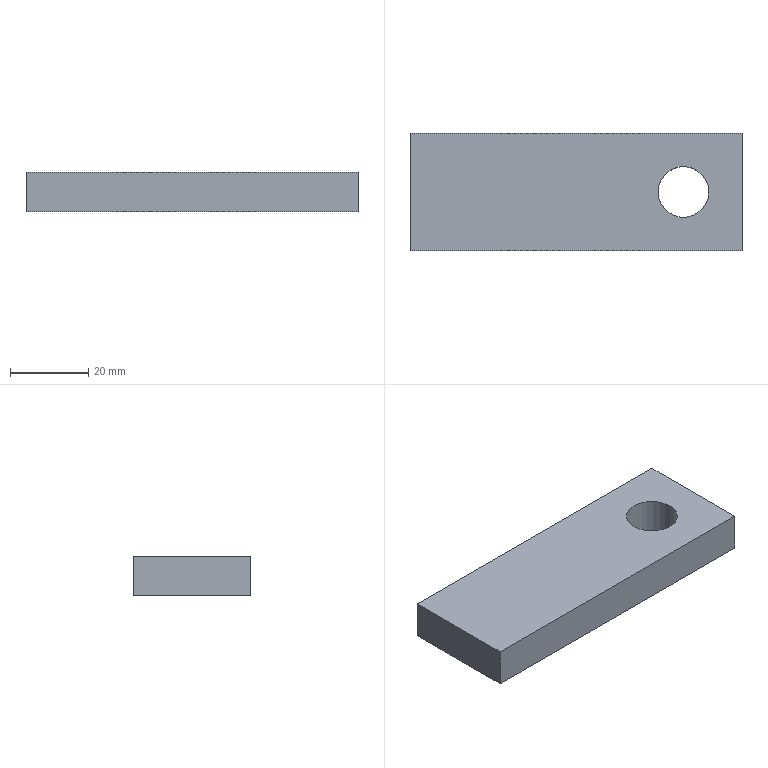Part | NX | features solid 2 | 1 solid | 7 faces | box 85 x 30 x 10 mm | volume 24173 mm3 | plane 6 | cylinder 1 | commonest cylinder face diameters 13 x1
STEP:
#1=CARTESIAN_POINT('',(-510.,-55.,-65.));
#2=VERTEX_POINT('',#1);
#3=CARTESIAN_POINT('',(-510.,-55.,-55.));
#4=VERTEX_POINT('',#3);
#5=CARTESIAN_POINT('',(-510.,-55.,0.));
#6=DIRECTION('',(0.,0.,-1.));
#7=VECTOR('',#6,1000.);
#8=LINE('',#5,#7);
#9=EDGE_CURVE('',#2,#4,#8,.F.);
#10=ORIENTED_EDGE('',*,*,#9,.T.);
#11=CARTESIAN_POINT('',(-595.,-55.,-55.));
#12=VERTEX_POINT('',#11);
#13=CARTESIAN_POINT('',(-610.,-55.,-55.));
#14=DIRECTION('',(-1.,0.,0.));
#15=VECTOR('',#14,1000.);
#16=LINE('',#13,#15);
#17=EDGE_CURVE('',#4,#12,#16,.T.);
#18=ORIENTED_EDGE('',*,*,#17,.T.);
#19=CARTESIAN_POINT('',(-595.,-55.,-65.));
#20=VERTEX_POINT('',#19);
#21=CARTESIAN_POINT('',(-595.,-55.,-65.));
#22=DIRECTION('',(0.,0.,-1.));
#23=VECTOR('',#22,1000.);
#24=LINE('',#21,#23);
#25=EDGE_CURVE('',#12,#20,#24,.T.);
#26=ORIENTED_EDGE('',*,*,#25,.T.);
#27=CARTESIAN_POINT('',(-610.,-55.,-65.));
#28=DIRECTION('',(-1.,0.,0.));
#29=VECTOR('',#28,1000.);
#30=LINE('',#27,#29);
#31=EDGE_CURVE('',#20,#2,#30,.F.);
#32=ORIENTED_EDGE('',*,*,#31,.T.);
#33=EDGE_LOOP('',(#10,#18,#26,#32));
#34=FACE_BOUND('',#33,.T.);
#35=CARTESIAN_POINT('',(-525.,-55.,0.));
#36=DIRECTION('',(0.,-1.,0.));
#37=DIRECTION('',(0.,0.,-1.));
#38=AXIS2_PLACEMENT_3D('',#35,#36,#37);
#39=PLANE('',#38);
#40=ADVANCED_FACE('',(#34),#39,.T.);
#41=CARTESIAN_POINT('',(-531.5,-40.,-55.));
#42=VERTEX_POINT('',#41);
#43=CARTESIAN_POINT('',(-525.,-40.,-55.));
#44=DIRECTION('',(0.,0.,-1.));
#45=DIRECTION('',(-1.,0.,0.));
#46=AXIS2_PLACEMENT_3D('',#43,#44,#45);
#47=CIRCLE('',#46,6.5);
#48=EDGE_CURVE('',#42,#42,#47,.T.);
#49=ORIENTED_EDGE('',*,*,#48,.F.);
#50=EDGE_LOOP('',(#49));
#51=FACE_BOUND('',#50,.T.);
#52=CARTESIAN_POINT('',(-531.5,-40.,-65.));
#53=VERTEX_POINT('',#52);
#54=CARTESIAN_POINT('',(-525.,-40.,-65.));
#55=DIRECTION('',(0.,0.,-1.));
#56=DIRECTION('',(-1.,0.,0.));
#57=AXIS2_PLACEMENT_3D('',#54,#55,#56);
#58=CIRCLE('',#57,6.5);
#59=EDGE_CURVE('',#53,#53,#58,.F.);
#60=ORIENTED_EDGE('',*,*,#59,.F.);
#61=EDGE_LOOP('',(#60));
#62=FACE_BOUND('',#61,.T.);
#63=CARTESIAN_POINT('',(-525.,-40.,-55.));
#64=DIRECTION('',(0.,0.,-1.));
#65=DIRECTION('',(-1.,0.,0.));
#66=AXIS2_PLACEMENT_3D('',#63,#64,#65);
#67=CYLINDRICAL_SURFACE('',#66,6.5);
#68=ADVANCED_FACE('',(#51,#62),#67,.F.);
#69=CARTESIAN_POINT('',(-595.,-25.,-65.));
#70=VERTEX_POINT('',#69);
#71=CARTESIAN_POINT('',(-510.,-25.,-65.));
#72=VERTEX_POINT('',#71);
#73=CARTESIAN_POINT('',(-610.,-25.,-65.));
#74=DIRECTION('',(-1.,0.,0.));
#75=VECTOR('',#74,1000.);
#76=LINE('',#73,#75);
#77=EDGE_CURVE('',#70,#72,#76,.F.);
#78=ORIENTED_EDGE('',*,*,#77,.F.);
#79=CARTESIAN_POINT('',(-595.,-25.,-55.));
#80=VERTEX_POINT('',#79);
#81=CARTESIAN_POINT('',(-595.,-25.,-65.));
#82=DIRECTION('',(0.,0.,1.));
#83=VECTOR('',#82,1000.);
#84=LINE('',#81,#83);
#85=EDGE_CURVE('',#70,#80,#84,.T.);
#86=ORIENTED_EDGE('',*,*,#85,.T.);
#87=CARTESIAN_POINT('',(-510.,-25.,-55.));
#88=VERTEX_POINT('',#87);
#89=CARTESIAN_POINT('',(-610.,-25.,-55.));
#90=DIRECTION('',(-1.,0.,0.));
#91=VECTOR('',#90,1000.);
#92=LINE('',#89,#91);
#93=EDGE_CURVE('',#88,#80,#92,.T.);
#94=ORIENTED_EDGE('',*,*,#93,.F.);
#95=CARTESIAN_POINT('',(-510.,-25.,0.));
#96=DIRECTION('',(0.,0.,1.));
#97=VECTOR('',#96,1000.);
#98=LINE('',#95,#97);
#99=EDGE_CURVE('',#88,#72,#98,.F.);
#100=ORIENTED_EDGE('',*,*,#99,.T.);
#101=EDGE_LOOP('',(#78,#86,#94,#100));
#102=FACE_BOUND('',#101,.T.);
#103=CARTESIAN_POINT('',(-525.,-25.,0.));
#104=DIRECTION('',(0.,-1.,0.));
#105=DIRECTION('',(0.,0.,-1.));
#106=AXIS2_PLACEMENT_3D('',#103,#104,#105);
#107=PLANE('',#106);
#108=ADVANCED_FACE('',(#102),#107,.F.);
#109=ORIENTED_EDGE('',*,*,#85,.F.);
#110=CARTESIAN_POINT('',(-595.,110.,-65.));
#111=DIRECTION('',(0.,1.,0.));
#112=VECTOR('',#111,1000.);
#113=LINE('',#110,#112);
#114=EDGE_CURVE('',#20,#70,#113,.T.);
#115=ORIENTED_EDGE('',*,*,#114,.F.);
#116=ORIENTED_EDGE('',*,*,#25,.F.);
#117=CARTESIAN_POINT('',(-595.,110.,-55.));
#118=DIRECTION('',(0.,1.,0.));
#119=VECTOR('',#118,1000.);
#120=LINE('',#117,#119);
#121=EDGE_CURVE('',#12,#80,#120,.T.);
#122=ORIENTED_EDGE('',*,*,#121,.T.);
#123=EDGE_LOOP('',(#109,#115,#116,#122));
#124=FACE_BOUND('',#123,.T.);
#125=CARTESIAN_POINT('',(-595.,110.,-65.));
#126=DIRECTION('',(1.,0.,0.));
#127=DIRECTION('',(0.,0.,-1.));
#128=AXIS2_PLACEMENT_3D('',#125,#126,#127);
#129=PLANE('',#128);
#130=ADVANCED_FACE('',(#124),#129,.F.);
#131=ORIENTED_EDGE('',*,*,#9,.F.);
#132=CARTESIAN_POINT('',(-510.,90.,-65.));
#133=DIRECTION('',(0.,1.,0.));
#134=VECTOR('',#133,1000.);
#135=LINE('',#132,#134);
#136=EDGE_CURVE('',#72,#2,#135,.F.);
#137=ORIENTED_EDGE('',*,*,#136,.F.);
#138=ORIENTED_EDGE('',*,*,#99,.F.);
#139=CARTESIAN_POINT('',(-510.,-25.,-55.));
#140=DIRECTION('',(0.,1.,0.));
#141=VECTOR('',#140,1000.);
#142=LINE('',#139,#141);
#143=EDGE_CURVE('',#88,#4,#142,.F.);
#144=ORIENTED_EDGE('',*,*,#143,.T.);
#145=EDGE_LOOP('',(#131,#137,#138,#144));
#146=FACE_BOUND('',#145,.T.);
#147=CARTESIAN_POINT('',(-510.,90.,0.));
#148=DIRECTION('',(1.,0.,0.));
#149=DIRECTION('',(0.,0.,-1.));
#150=AXIS2_PLACEMENT_3D('',#147,#148,#149);
#151=PLANE('',#150);
#152=ADVANCED_FACE('',(#146),#151,.T.);
#153=ORIENTED_EDGE('',*,*,#59,.T.);
#154=EDGE_LOOP('',(#153));
#155=FACE_BOUND('',#154,.T.);
#156=ORIENTED_EDGE('',*,*,#31,.F.);
#157=ORIENTED_EDGE('',*,*,#114,.T.);
#158=ORIENTED_EDGE('',*,*,#77,.T.);
#159=ORIENTED_EDGE('',*,*,#136,.T.);
#160=EDGE_LOOP('',(#156,#157,#158,#159));
#161=FACE_BOUND('',#160,.T.);
#162=CARTESIAN_POINT('',(-610.,110.,-65.));
#163=DIRECTION('',(0.,0.,-1.));
#164=DIRECTION('',(0.,1.,0.));
#165=AXIS2_PLACEMENT_3D('',#162,#163,#164);
#166=PLANE('',#165);
#167=ADVANCED_FACE('',(#155,#161),#166,.T.);
#168=ORIENTED_EDGE('',*,*,#48,.T.);
#169=EDGE_LOOP('',(#168));
#170=FACE_BOUND('',#169,.T.);
#171=ORIENTED_EDGE('',*,*,#17,.F.);
#172=ORIENTED_EDGE('',*,*,#143,.F.);
#173=ORIENTED_EDGE('',*,*,#93,.T.);
#174=ORIENTED_EDGE('',*,*,#121,.F.);
#175=EDGE_LOOP('',(#171,#172,#173,#174));
#176=FACE_BOUND('',#175,.T.);
#177=CARTESIAN_POINT('',(-610.,110.,-55.));
#178=DIRECTION('',(0.,0.,-1.));
#179=DIRECTION('',(0.,1.,0.));
#180=AXIS2_PLACEMENT_3D('',#177,#178,#179);
#181=PLANE('',#180);
#182=ADVANCED_FACE('',(#170,#176),#181,.F.);
#183=CLOSED_SHELL('',(#40,#68,#108,#130,#152,#167,#182));
#184=MANIFOLD_SOLID_BREP('',#183);
#185=(LENGTH_UNIT()NAMED_UNIT(*)SI_UNIT(.MILLI.,.METRE.));
#186=UNCERTAINTY_MEASURE_WITH_UNIT(LENGTH_MEASURE(0.00001),#185,'','');
#187=(NAMED_UNIT(*)PLANE_ANGLE_UNIT()SI_UNIT($,.RADIAN.));
#188=(NAMED_UNIT(*)SI_UNIT($,.STERADIAN.)SOLID_ANGLE_UNIT());
#189=(GEOMETRIC_REPRESENTATION_CONTEXT(3)GLOBAL_UNCERTAINTY_ASSIGNED_CONTEXT((#186))GLOBAL_UNIT_ASSIGNED_CONTEXT((#185,#187,#188))REPRESENTATION_CONTEXT('',''));
#190=ADVANCED_BREP_SHAPE_REPRESENTATION('',(#184),#189);